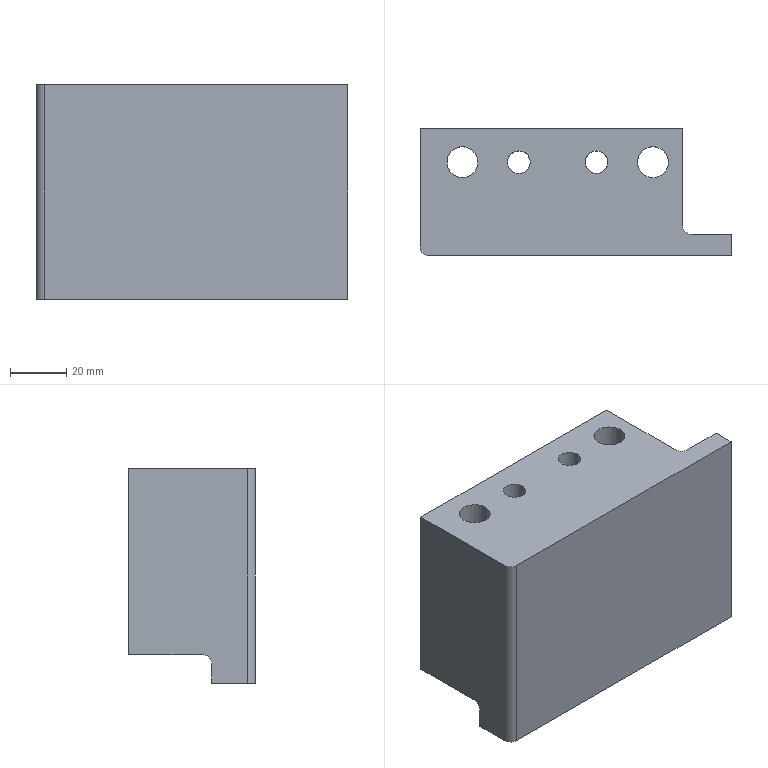Part | NX | features solid 2 | 1 solid | 25 faces | box 110.531 x 45 x 76 mm | volume 269432 mm3 | plane 14 | cylinder 11 | commonest cylinder face diameters 6 x3 8 x2 10.505 x2 11 x2 17 x2
STEP:
#1=CARTESIAN_POINT('',(682.498,166.969,32.999));
#2=VERTEX_POINT('',#1);
#3=CARTESIAN_POINT('',(682.498,201.487,32.999));
#4=VERTEX_POINT('',#3);
#5=CARTESIAN_POINT('',(682.498,196.487,32.999));
#6=DIRECTION('',(0.,-1.,-0.000000517));
#7=VECTOR('',#6,1000.);
#8=LINE('',#5,#7);
#9=EDGE_CURVE('',#2,#4,#8,.F.);
#10=ORIENTED_EDGE('',*,*,#9,.F.);
#11=CARTESIAN_POINT('',(682.498,166.969,-33.001));
#12=VERTEX_POINT('',#11);
#13=CARTESIAN_POINT('',(682.498,166.969,-43.001));
#14=DIRECTION('',(0.,0.000004945,-1.));
#15=VECTOR('',#14,1000.);
#16=LINE('',#13,#15);
#17=EDGE_CURVE('',#2,#12,#16,.T.);
#18=ORIENTED_EDGE('',*,*,#17,.T.);
#19=CARTESIAN_POINT('',(682.498,166.969,-43.001));
#20=VERTEX_POINT('',#19);
#21=CARTESIAN_POINT('',(682.498,166.969,-33.001));
#22=CARTESIAN_POINT('',(682.498,166.969,-36.334));
#23=CARTESIAN_POINT('',(682.498,166.969,-39.668));
#24=CARTESIAN_POINT('',(682.498,166.969,-43.001));
#25=B_SPLINE_CURVE_WITH_KNOTS('',3,(#21,#22,#23,#24),.UNSPECIFIED.,.F.,.F.,(4,4),(0.,1.),.UNSPECIFIED.);
#26=EDGE_CURVE('',#12,#20,#25,.T.);
#27=ORIENTED_EDGE('',*,*,#26,.T.);
#28=CARTESIAN_POINT('',(682.498,171.969,-43.001));
#29=VERTEX_POINT('',#28);
#30=CARTESIAN_POINT('',(682.498,166.969,-43.001));
#31=CARTESIAN_POINT('',(682.498,168.636,-43.001));
#32=CARTESIAN_POINT('',(682.498,170.302,-43.001));
#33=CARTESIAN_POINT('',(682.498,171.969,-43.001));
#34=B_SPLINE_CURVE_WITH_KNOTS('',3,(#30,#31,#32,#33),.UNSPECIFIED.,.F.,.F.,(4,4),(0.,1.),.UNSPECIFIED.);
#35=EDGE_CURVE('',#29,#20,#34,.F.);
#36=ORIENTED_EDGE('',*,*,#35,.F.);
#37=CARTESIAN_POINT('',(682.498,171.969,-36.001));
#38=VERTEX_POINT('',#37);
#39=CARTESIAN_POINT('',(682.498,171.969,-43.001));
#40=CARTESIAN_POINT('',(682.498,171.969,-40.668));
#41=CARTESIAN_POINT('',(682.498,171.969,-38.334));
#42=CARTESIAN_POINT('',(682.498,171.969,-36.001));
#43=B_SPLINE_CURVE_WITH_KNOTS('',3,(#39,#40,#41,#42),.UNSPECIFIED.,.F.,.F.,(4,4),(0.,0.7),.UNSPECIFIED.);
#44=EDGE_CURVE('',#38,#29,#43,.F.);
#45=ORIENTED_EDGE('',*,*,#44,.F.);
#46=CARTESIAN_POINT('',(682.498,174.969,-33.001));
#47=VERTEX_POINT('',#46);
#48=CARTESIAN_POINT('',(682.498,174.969,-36.001));
#49=DIRECTION('',(1.,0.,0.));
#50=DIRECTION('',(0.,1.,0.));
#51=AXIS2_PLACEMENT_3D('',#48,#49,#50);
#52=CIRCLE('',#51,3.);
#53=EDGE_CURVE('',#38,#47,#52,.F.);
#54=ORIENTED_EDGE('',*,*,#53,.T.);
#55=CARTESIAN_POINT('',(682.498,201.487,-33.001));
#56=VERTEX_POINT('',#55);
#57=CARTESIAN_POINT('',(682.498,119.199,-33.001));
#58=DIRECTION('',(0.,-1.,-0.000000517));
#59=VECTOR('',#58,1000.);
#60=LINE('',#57,#59);
#61=EDGE_CURVE('',#47,#56,#60,.F.);
#62=ORIENTED_EDGE('',*,*,#61,.T.);
#63=CARTESIAN_POINT('',(682.498,201.487,-43.001));
#64=DIRECTION('',(0.,-0.000000517,1.));
#65=VECTOR('',#64,1000.);
#66=LINE('',#63,#65);
#67=EDGE_CURVE('',#56,#4,#66,.T.);
#68=ORIENTED_EDGE('',*,*,#67,.T.);
#69=EDGE_LOOP('',(#10,#18,#27,#36,#45,#54,#62,#68));
#70=FACE_BOUND('',#69,.T.);
#71=CARTESIAN_POINT('',(682.498,185.969,49.2));
#72=DIRECTION('',(1.,0.,0.));
#73=DIRECTION('',(0.,-1.,-0.000004363));
#74=AXIS2_PLACEMENT_3D('',#71,#72,#73);
#75=PLANE('',#74);
#76=ADVANCED_FACE('',(#70),#75,.T.);
#77=CARTESIAN_POINT('',(671.977,197.987,-33.001));
#78=VERTEX_POINT('',#77);
#79=CARTESIAN_POINT('',(671.977,189.487,-33.001));
#80=DIRECTION('',(-0.000000053,0.000000517,-1.));
#81=DIRECTION('',(0.,1.,0.000000517));
#82=AXIS2_PLACEMENT_3D('',#79,#80,#81);
#83=CIRCLE('',#82,8.5);
#84=EDGE_CURVE('',#78,#78,#83,.F.);
#85=ORIENTED_EDGE('',*,*,#84,.T.);
#86=EDGE_LOOP('',(#85));
#87=FACE_BOUND('',#86,.T.);
#88=CARTESIAN_POINT('',(651.977,194.739,-33.001));
#89=VERTEX_POINT('',#88);
#90=CARTESIAN_POINT('',(651.977,189.487,-33.001));
#91=DIRECTION('',(-0.000000053,0.000000517,-1.));
#92=DIRECTION('',(0.,1.,0.000000517));
#93=AXIS2_PLACEMENT_3D('',#90,#91,#92);
#94=CIRCLE('',#93,5.253);
#95=EDGE_CURVE('',#89,#89,#94,.F.);
#96=ORIENTED_EDGE('',*,*,#95,.T.);
#97=EDGE_LOOP('',(#96));
#98=FACE_BOUND('',#97,.T.);
#99=CARTESIAN_POINT('',(624.446,194.739,-33.001));
#100=VERTEX_POINT('',#99);
#101=CARTESIAN_POINT('',(624.446,189.487,-33.001));
#102=DIRECTION('',(-0.000000053,0.000000517,-1.));
#103=DIRECTION('',(0.,1.,0.000000517));
#104=AXIS2_PLACEMENT_3D('',#101,#102,#103);
#105=CIRCLE('',#104,5.253);
#106=EDGE_CURVE('',#100,#100,#105,.F.);
#107=ORIENTED_EDGE('',*,*,#106,.T.);
#108=EDGE_LOOP('',(#107));
#109=FACE_BOUND('',#108,.T.);
#110=CARTESIAN_POINT('',(604.446,197.987,-33.001));
#111=VERTEX_POINT('',#110);
#112=CARTESIAN_POINT('',(604.446,189.487,-33.001));
#113=DIRECTION('',(-0.000000053,0.000000517,-1.));
#114=DIRECTION('',(0.,1.,0.000000517));
#115=AXIS2_PLACEMENT_3D('',#112,#113,#114);
#116=CIRCLE('',#115,8.5);
#117=EDGE_CURVE('',#111,#111,#116,.F.);
#118=ORIENTED_EDGE('',*,*,#117,.T.);
#119=EDGE_LOOP('',(#118));
#120=FACE_BOUND('',#119,.T.);
#121=ORIENTED_EDGE('',*,*,#61,.F.);
#122=CARTESIAN_POINT('',(589.446,174.969,-33.001));
#123=VERTEX_POINT('',#122);
#124=CARTESIAN_POINT('',(589.446,174.969,-33.001));
#125=DIRECTION('',(1.,0.,-0.000000053));
#126=VECTOR('',#125,1000.);
#127=LINE('',#124,#126);
#128=EDGE_CURVE('',#47,#123,#127,.F.);
#129=ORIENTED_EDGE('',*,*,#128,.T.);
#130=CARTESIAN_POINT('',(589.446,201.487,-33.001));
#131=VERTEX_POINT('',#130);
#132=CARTESIAN_POINT('',(589.446,119.199,-33.001));
#133=DIRECTION('',(0.,-1.,-0.000000517));
#134=VECTOR('',#133,1000.);
#135=LINE('',#132,#134);
#136=EDGE_CURVE('',#131,#123,#135,.T.);
#137=ORIENTED_EDGE('',*,*,#136,.F.);
#138=CARTESIAN_POINT('',(574.977,201.487,-33.001));
#139=DIRECTION('',(-1.,0.,0.000000053));
#140=VECTOR('',#139,1000.);
#141=LINE('',#138,#140);
#142=EDGE_CURVE('',#56,#131,#141,.T.);
#143=ORIENTED_EDGE('',*,*,#142,.F.);
#144=EDGE_LOOP('',(#121,#129,#137,#143));
#145=FACE_BOUND('',#144,.T.);
#146=CARTESIAN_POINT('',(574.977,119.199,-33.001));
#147=DIRECTION('',(-0.000000053,0.000000517,-1.));
#148=DIRECTION('',(1.,0.,-0.000000053));
#149=AXIS2_PLACEMENT_3D('',#146,#147,#148);
#150=PLANE('',#149);
#151=ADVANCED_FACE('',(#87,#98,#109,#120,#145),#150,.T.);
#152=CARTESIAN_POINT('',(699.977,163.969,32.999));
#153=VERTEX_POINT('',#152);
#154=CARTESIAN_POINT('',(685.498,163.969,32.999));
#155=VERTEX_POINT('',#154);
#156=CARTESIAN_POINT('',(704.737,163.969,32.999));
#157=DIRECTION('',(1.,0.,-0.000000053));
#158=VECTOR('',#157,1000.);
#159=LINE('',#156,#158);
#160=EDGE_CURVE('',#153,#155,#159,.F.);
#161=ORIENTED_EDGE('',*,*,#160,.T.);
#162=CARTESIAN_POINT('',(685.498,166.969,32.999));
#163=DIRECTION('',(0.000000053,-0.000000517,1.));
#164=DIRECTION('',(-0.01202,-0.9999,-0.000000516));
#165=AXIS2_PLACEMENT_3D('',#162,#163,#164);
#166=ELLIPSE('',#165,3.,3.);
#167=EDGE_CURVE('',#155,#2,#166,.F.);
#168=ORIENTED_EDGE('',*,*,#167,.T.);
#169=ORIENTED_EDGE('',*,*,#9,.T.);
#170=CARTESIAN_POINT('',(589.446,201.487,32.999));
#171=VERTEX_POINT('',#170);
#172=CARTESIAN_POINT('',(699.977,201.487,32.999));
#173=DIRECTION('',(-1.,0.,0.000000053));
#174=VECTOR('',#173,1000.);
#175=LINE('',#172,#174);
#176=EDGE_CURVE('',#171,#4,#175,.F.);
#177=ORIENTED_EDGE('',*,*,#176,.F.);
#178=CARTESIAN_POINT('',(589.446,159.487,32.999));
#179=VERTEX_POINT('',#178);
#180=CARTESIAN_POINT('',(589.446,186.487,32.999));
#181=DIRECTION('',(0.,-1.,-0.000000517));
#182=VECTOR('',#181,1000.);
#183=LINE('',#180,#182);
#184=EDGE_CURVE('',#179,#171,#183,.F.);
#185=ORIENTED_EDGE('',*,*,#184,.F.);
#186=CARTESIAN_POINT('',(592.446,156.487,32.999));
#187=VERTEX_POINT('',#186);
#188=CARTESIAN_POINT('',(592.446,159.487,32.999));
#189=DIRECTION('',(-0.000000053,0.000000517,-1.));
#190=DIRECTION('',(0.,-1.,-0.000000517));
#191=AXIS2_PLACEMENT_3D('',#188,#189,#190);
#192=CIRCLE('',#191,3.);
#193=EDGE_CURVE('',#179,#187,#192,.F.);
#194=ORIENTED_EDGE('',*,*,#193,.T.);
#195=CARTESIAN_POINT('',(699.977,156.487,32.999));
#196=VERTEX_POINT('',#195);
#197=CARTESIAN_POINT('',(699.977,156.487,32.999));
#198=DIRECTION('',(-1.,0.,0.000000053));
#199=VECTOR('',#198,1000.);
#200=LINE('',#197,#199);
#201=EDGE_CURVE('',#187,#196,#200,.F.);
#202=ORIENTED_EDGE('',*,*,#201,.T.);
#203=CARTESIAN_POINT('',(699.977,196.487,32.999));
#204=DIRECTION('',(0.,-1.,-0.000000517));
#205=VECTOR('',#204,1000.);
#206=LINE('',#203,#205);
#207=EDGE_CURVE('',#153,#196,#206,.T.);
#208=ORIENTED_EDGE('',*,*,#207,.F.);
#209=EDGE_LOOP('',(#161,#168,#169,#177,#185,#194,#202,#208));
#210=FACE_BOUND('',#209,.T.);
#211=CARTESIAN_POINT('',(671.977,183.987,32.999));
#212=VERTEX_POINT('',#211);
#213=CARTESIAN_POINT('',(671.977,189.487,32.999));
#214=DIRECTION('',(0.000000053,-0.000000517,1.));
#215=DIRECTION('',(0.,-1.,-0.000000517));
#216=AXIS2_PLACEMENT_3D('',#213,#214,#215);
#217=CIRCLE('',#216,5.5);
#218=EDGE_CURVE('',#212,#212,#217,.T.);
#219=ORIENTED_EDGE('',*,*,#218,.F.);
#220=EDGE_LOOP('',(#219));
#221=FACE_BOUND('',#220,.T.);
#222=CARTESIAN_POINT('',(651.977,193.487,32.999));
#223=VERTEX_POINT('',#222);
#224=CARTESIAN_POINT('',(651.977,189.487,32.999));
#225=DIRECTION('',(0.000000053,-0.000000517,1.));
#226=DIRECTION('',(0.,1.,0.000000517));
#227=AXIS2_PLACEMENT_3D('',#224,#225,#226);
#228=CIRCLE('',#227,4.);
#229=EDGE_CURVE('',#223,#223,#228,.T.);
#230=ORIENTED_EDGE('',*,*,#229,.F.);
#231=EDGE_LOOP('',(#230));
#232=FACE_BOUND('',#231,.T.);
#233=CARTESIAN_POINT('',(624.446,193.487,32.999));
#234=VERTEX_POINT('',#233);
#235=CARTESIAN_POINT('',(624.446,189.487,32.999));
#236=DIRECTION('',(0.000000053,-0.000000517,1.));
#237=DIRECTION('',(0.,1.,0.000000517));
#238=AXIS2_PLACEMENT_3D('',#235,#236,#237);
#239=CIRCLE('',#238,4.);
#240=EDGE_CURVE('',#234,#234,#239,.T.);
#241=ORIENTED_EDGE('',*,*,#240,.F.);
#242=EDGE_LOOP('',(#241));
#243=FACE_BOUND('',#242,.T.);
#244=CARTESIAN_POINT('',(604.446,183.987,32.999));
#245=VERTEX_POINT('',#244);
#246=CARTESIAN_POINT('',(604.446,189.487,32.999));
#247=DIRECTION('',(0.000000053,-0.000000517,1.));
#248=DIRECTION('',(0.,-1.,-0.000000517));
#249=AXIS2_PLACEMENT_3D('',#246,#247,#248);
#250=CIRCLE('',#249,5.5);
#251=EDGE_CURVE('',#245,#245,#250,.T.);
#252=ORIENTED_EDGE('',*,*,#251,.F.);
#253=EDGE_LOOP('',(#252));
#254=FACE_BOUND('',#253,.T.);
#255=CARTESIAN_POINT('',(699.977,196.487,32.999));
#256=DIRECTION('',(0.000000053,-0.000000517,1.));
#257=DIRECTION('',(1.,0.,-0.000000053));
#258=AXIS2_PLACEMENT_3D('',#255,#256,#257);
#259=PLANE('',#258);
#260=ADVANCED_FACE('',(#210,#221,#232,#243,#254),#259,.T.);
#261=CARTESIAN_POINT('',(589.446,171.969,-36.001));
#262=VERTEX_POINT('',#261);
#263=CARTESIAN_POINT('',(589.446,171.969,-43.001));
#264=VERTEX_POINT('',#263);
#265=CARTESIAN_POINT('',(589.446,171.969,-43.001));
#266=DIRECTION('',(-0.000000053,0.000001782,-1.));
#267=VECTOR('',#266,1000.);
#268=LINE('',#265,#267);
#269=EDGE_CURVE('',#262,#264,#268,.T.);
#270=ORIENTED_EDGE('',*,*,#269,.F.);
#271=CARTESIAN_POINT('',(682.498,171.969,-36.001));
#272=DIRECTION('',(1.,0.,-0.000000053));
#273=VECTOR('',#272,1000.);
#274=LINE('',#271,#273);
#275=EDGE_CURVE('',#262,#38,#274,.T.);
#276=ORIENTED_EDGE('',*,*,#275,.T.);
#277=ORIENTED_EDGE('',*,*,#44,.T.);
#278=CARTESIAN_POINT('',(704.737,171.969,-43.001));
#279=DIRECTION('',(-1.,0.,0.000000053));
#280=VECTOR('',#279,1000.);
#281=LINE('',#278,#280);
#282=EDGE_CURVE('',#29,#264,#281,.T.);
#283=ORIENTED_EDGE('',*,*,#282,.T.);
#284=EDGE_LOOP('',(#270,#276,#277,#283));
#285=FACE_BOUND('',#284,.T.);
#286=CARTESIAN_POINT('',(704.737,171.969,-5.001));
#287=DIRECTION('',(0.,1.,0.000001782));
#288=DIRECTION('',(0.,0.000001782,-1.));
#289=AXIS2_PLACEMENT_3D('',#286,#287,#288);
#290=PLANE('',#289);
#291=ADVANCED_FACE('',(#285),#290,.T.);
#292=CARTESIAN_POINT('',(592.446,156.487,-43.001));
#293=VERTEX_POINT('',#292);
#294=CARTESIAN_POINT('',(699.977,156.487,-43.001));
#295=VERTEX_POINT('',#294);
#296=CARTESIAN_POINT('',(574.977,156.487,-43.001));
#297=DIRECTION('',(1.,0.,-0.000000053));
#298=VECTOR('',#297,1000.);
#299=LINE('',#296,#298);
#300=EDGE_CURVE('',#293,#295,#299,.T.);
#301=ORIENTED_EDGE('',*,*,#300,.T.);
#302=CARTESIAN_POINT('',(699.977,156.487,56.368));
#303=DIRECTION('',(0.000000053,-0.000000517,1.));
#304=VECTOR('',#303,1000.);
#305=LINE('',#302,#304);
#306=EDGE_CURVE('',#295,#196,#305,.T.);
#307=ORIENTED_EDGE('',*,*,#306,.T.);
#308=ORIENTED_EDGE('',*,*,#201,.F.);
#309=CARTESIAN_POINT('',(592.446,156.487,56.368));
#310=DIRECTION('',(-0.000000053,0.000000517,-1.));
#311=VECTOR('',#310,1000.);
#312=LINE('',#309,#311);
#313=EDGE_CURVE('',#187,#293,#312,.T.);
#314=ORIENTED_EDGE('',*,*,#313,.T.);
#315=EDGE_LOOP('',(#301,#307,#308,#314));
#316=FACE_BOUND('',#315,.T.);
#317=CARTESIAN_POINT('',(583.446,156.487,56.368));
#318=DIRECTION('',(0.,1.,0.000000517));
#319=DIRECTION('',(-0.000000053,0.000000517,-1.));
#320=AXIS2_PLACEMENT_3D('',#317,#318,#319);
#321=PLANE('',#320);
#322=ADVANCED_FACE('',(#316),#321,.F.);
#323=ORIENTED_EDGE('',*,*,#282,.F.);
#324=ORIENTED_EDGE('',*,*,#35,.T.);
#325=CARTESIAN_POINT('',(685.498,163.969,-43.001));
#326=VERTEX_POINT('',#325);
#327=CARTESIAN_POINT('',(685.498,166.969,-43.001));
#328=DIRECTION('',(-0.000000053,0.000000517,-1.));
#329=DIRECTION('',(-0.01202,-0.9999,-0.000000516));
#330=AXIS2_PLACEMENT_3D('',#327,#328,#329);
#331=ELLIPSE('',#330,3.,3.);
#332=EDGE_CURVE('',#20,#326,#331,.F.);
#333=ORIENTED_EDGE('',*,*,#332,.T.);
#334=CARTESIAN_POINT('',(699.977,163.969,-43.001));
#335=VERTEX_POINT('',#334);
#336=CARTESIAN_POINT('',(704.737,163.969,-43.001));
#337=DIRECTION('',(-1.,0.,0.000000053));
#338=VECTOR('',#337,1000.);
#339=LINE('',#336,#338);
#340=EDGE_CURVE('',#335,#326,#339,.T.);
#341=ORIENTED_EDGE('',*,*,#340,.F.);
#342=CARTESIAN_POINT('',(699.977,119.199,-43.001));
#343=DIRECTION('',(0.,1.,0.000000517));
#344=VECTOR('',#343,1000.);
#345=LINE('',#342,#344);
#346=EDGE_CURVE('',#295,#335,#345,.T.);
#347=ORIENTED_EDGE('',*,*,#346,.F.);
#348=ORIENTED_EDGE('',*,*,#300,.F.);
#349=CARTESIAN_POINT('',(589.446,159.487,-43.001));
#350=VERTEX_POINT('',#349);
#351=CARTESIAN_POINT('',(592.446,159.487,-43.001));
#352=DIRECTION('',(0.000000053,-0.000000517,1.));
#353=DIRECTION('',(0.,1.,0.000000517));
#354=AXIS2_PLACEMENT_3D('',#351,#352,#353);
#355=CIRCLE('',#354,3.);
#356=EDGE_CURVE('',#293,#350,#355,.F.);
#357=ORIENTED_EDGE('',*,*,#356,.T.);
#358=CARTESIAN_POINT('',(589.446,119.199,-43.001));
#359=DIRECTION('',(0.,-1.,-0.000000517));
#360=VECTOR('',#359,1000.);
#361=LINE('',#358,#360);
#362=EDGE_CURVE('',#264,#350,#361,.T.);
#363=ORIENTED_EDGE('',*,*,#362,.F.);
#364=EDGE_LOOP('',(#323,#324,#333,#341,#347,#348,#357,#363));
#365=FACE_BOUND('',#364,.T.);
#366=CARTESIAN_POINT('',(574.977,119.199,-43.001));
#367=DIRECTION('',(-0.000000053,0.000000517,-1.));
#368=DIRECTION('',(1.,0.,-0.000000053));
#369=AXIS2_PLACEMENT_3D('',#366,#367,#368);
#370=PLANE('',#369);
#371=ADVANCED_FACE('',(#365),#370,.T.);
#372=ORIENTED_EDGE('',*,*,#142,.T.);
#373=CARTESIAN_POINT('',(589.446,201.487,-43.001));
#374=DIRECTION('',(0.000000053,-0.000000517,1.));
#375=VECTOR('',#374,1000.);
#376=LINE('',#373,#375);
#377=EDGE_CURVE('',#171,#131,#376,.F.);
#378=ORIENTED_EDGE('',*,*,#377,.F.);
#379=ORIENTED_EDGE('',*,*,#176,.T.);
#380=ORIENTED_EDGE('',*,*,#67,.F.);
#381=EDGE_LOOP('',(#372,#378,#379,#380));
#382=FACE_BOUND('',#381,.T.);
#383=CARTESIAN_POINT('',(699.977,201.487,-43.001));
#384=DIRECTION('',(0.,1.,0.000000517));
#385=DIRECTION('',(-0.000000053,0.000000517,-1.));
#386=AXIS2_PLACEMENT_3D('',#383,#384,#385);
#387=PLANE('',#386);
#388=ADVANCED_FACE('',(#382),#387,.T.);
#389=ORIENTED_EDGE('',*,*,#136,.T.);
#390=CARTESIAN_POINT('',(589.446,174.969,-36.001));
#391=DIRECTION('',(-1.,0.,0.000000053));
#392=DIRECTION('',(0.000000053,0.,1.));
#393=AXIS2_PLACEMENT_3D('',#390,#391,#392);
#394=CIRCLE('',#393,3.);
#395=EDGE_CURVE('',#123,#262,#394,.F.);
#396=ORIENTED_EDGE('',*,*,#395,.T.);
#397=ORIENTED_EDGE('',*,*,#269,.T.);
#398=ORIENTED_EDGE('',*,*,#362,.T.);
#399=CARTESIAN_POINT('',(589.446,159.487,-43.001));
#400=DIRECTION('',(-0.000000053,0.000000517,-1.));
#401=VECTOR('',#400,1000.);
#402=LINE('',#399,#401);
#403=EDGE_CURVE('',#350,#179,#402,.F.);
#404=ORIENTED_EDGE('',*,*,#403,.T.);
#405=ORIENTED_EDGE('',*,*,#184,.T.);
#406=ORIENTED_EDGE('',*,*,#377,.T.);
#407=EDGE_LOOP('',(#389,#396,#397,#398,#404,#405,#406));
#408=FACE_BOUND('',#407,.T.);
#409=CARTESIAN_POINT('',(589.446,186.487,-43.001));
#410=DIRECTION('',(-1.,0.,0.000000053));
#411=DIRECTION('',(-0.000000053,0.000000517,-1.));
#412=AXIS2_PLACEMENT_3D('',#409,#410,#411);
#413=PLANE('',#412);
#414=ADVANCED_FACE('',(#408),#413,.T.);
#415=CARTESIAN_POINT('',(671.977,194.987,7.999));
#416=VERTEX_POINT('',#415);
#417=CARTESIAN_POINT('',(671.977,189.487,7.999));
#418=DIRECTION('',(-0.000000053,0.000000517,-1.));
#419=DIRECTION('',(0.,1.,0.000000517));
#420=AXIS2_PLACEMENT_3D('',#417,#418,#419);
#421=CIRCLE('',#420,5.5);
#422=EDGE_CURVE('',#416,#416,#421,.F.);
#423=ORIENTED_EDGE('',*,*,#422,.F.);
#424=EDGE_LOOP('',(#423));
#425=FACE_BOUND('',#424,.T.);
#426=ORIENTED_EDGE('',*,*,#218,.T.);
#427=EDGE_LOOP('',(#426));
#428=FACE_BOUND('',#427,.T.);
#429=CARTESIAN_POINT('',(671.977,189.487,33.999));
#430=DIRECTION('',(-0.000000053,0.000000517,-1.));
#431=DIRECTION('',(0.,1.,0.000000517));
#432=AXIS2_PLACEMENT_3D('',#429,#430,#431);
#433=CYLINDRICAL_SURFACE('',#432,5.5);
#434=ADVANCED_FACE('',(#425,#428),#433,.F.);
#435=ORIENTED_EDGE('',*,*,#84,.F.);
#436=EDGE_LOOP('',(#435));
#437=FACE_BOUND('',#436,.T.);
#438=CARTESIAN_POINT('',(671.977,197.987,7.999));
#439=VERTEX_POINT('',#438);
#440=CARTESIAN_POINT('',(671.977,189.487,7.999));
#441=DIRECTION('',(-0.000000053,0.000000517,-1.));
#442=DIRECTION('',(0.,1.,0.000000517));
#443=AXIS2_PLACEMENT_3D('',#440,#441,#442);
#444=CIRCLE('',#443,8.5);
#445=EDGE_CURVE('',#439,#439,#444,.T.);
#446=ORIENTED_EDGE('',*,*,#445,.F.);
#447=EDGE_LOOP('',(#446));
#448=FACE_BOUND('',#447,.T.);
#449=CARTESIAN_POINT('',(671.977,189.487,7.999));
#450=DIRECTION('',(-0.000000053,0.000000517,-1.));
#451=DIRECTION('',(0.,1.,0.000000517));
#452=AXIS2_PLACEMENT_3D('',#449,#450,#451);
#453=CYLINDRICAL_SURFACE('',#452,8.5);
#454=ADVANCED_FACE('',(#437,#448),#453,.F.);
#455=ORIENTED_EDGE('',*,*,#422,.T.);
#456=EDGE_LOOP('',(#455));
#457=FACE_BOUND('',#456,.T.);
#458=ORIENTED_EDGE('',*,*,#445,.T.);
#459=EDGE_LOOP('',(#458));
#460=FACE_BOUND('',#459,.T.);
#461=CARTESIAN_POINT('',(671.977,189.487,7.999));
#462=DIRECTION('',(-0.000000053,0.000000517,-1.));
#463=DIRECTION('',(0.,1.,0.000000517));
#464=AXIS2_PLACEMENT_3D('',#461,#462,#463);
#465=PLANE('',#464);
#466=ADVANCED_FACE('',(#457,#460),#465,.T.);
#467=CARTESIAN_POINT('',(655.977,189.487,-13.001));
#468=VERTEX_POINT('',#467);
#469=CARTESIAN_POINT('',(651.977,189.487,-13.001));
#470=DIRECTION('',(0.000000981,-0.000000517,-1.));
#471=DIRECTION('',(1.,0.,0.000000981));
#472=AXIS2_PLACEMENT_3D('',#469,#470,#471);
#473=CIRCLE('',#472,4.);
#474=EDGE_CURVE('',#468,#468,#473,.F.);
#475=ORIENTED_EDGE('',*,*,#474,.F.);
#476=EDGE_LOOP('',(#475));
#477=FACE_BOUND('',#476,.T.);
#478=ORIENTED_EDGE('',*,*,#229,.T.);
#479=EDGE_LOOP('',(#478));
#480=FACE_BOUND('',#479,.T.);
#481=CARTESIAN_POINT('',(651.977,189.487,33.999));
#482=DIRECTION('',(0.000000981,-0.000000517,-1.));
#483=DIRECTION('',(0.,1.,-0.000000517));
#484=AXIS2_PLACEMENT_3D('',#481,#482,#483);
#485=CYLINDRICAL_SURFACE('',#484,4.);
#486=ADVANCED_FACE('',(#477,#480),#485,.F.);
#487=ORIENTED_EDGE('',*,*,#95,.F.);
#488=EDGE_LOOP('',(#487));
#489=FACE_BOUND('',#488,.T.);
#490=CARTESIAN_POINT('',(657.23,189.487,-13.001));
#491=VERTEX_POINT('',#490);
#492=CARTESIAN_POINT('',(651.977,189.487,-13.001));
#493=DIRECTION('',(0.000000981,-0.000000517,-1.));
#494=DIRECTION('',(1.,0.,0.000000981));
#495=AXIS2_PLACEMENT_3D('',#492,#493,#494);
#496=CIRCLE('',#495,5.253);
#497=EDGE_CURVE('',#491,#491,#496,.T.);
#498=ORIENTED_EDGE('',*,*,#497,.F.);
#499=EDGE_LOOP('',(#498));
#500=FACE_BOUND('',#499,.T.);
#501=CARTESIAN_POINT('',(651.977,189.487,-33.001));
#502=DIRECTION('',(0.000000981,-0.000000517,-1.));
#503=DIRECTION('',(0.,1.,-0.000000517));
#504=AXIS2_PLACEMENT_3D('',#501,#502,#503);
#505=CYLINDRICAL_SURFACE('',#504,5.253);
#506=ADVANCED_FACE('',(#489,#500),#505,.F.);
#507=ORIENTED_EDGE('',*,*,#474,.T.);
#508=EDGE_LOOP('',(#507));
#509=FACE_BOUND('',#508,.T.);
#510=ORIENTED_EDGE('',*,*,#497,.T.);
#511=EDGE_LOOP('',(#510));
#512=FACE_BOUND('',#511,.T.);
#513=CARTESIAN_POINT('',(651.977,189.487,-13.001));
#514=DIRECTION('',(0.000000981,-0.000000517,-1.));
#515=DIRECTION('',(0.,1.,-0.000000517));
#516=AXIS2_PLACEMENT_3D('',#513,#514,#515);
#517=PLANE('',#516);
#518=ADVANCED_FACE('',(#509,#512),#517,.T.);
#519=CARTESIAN_POINT('',(624.446,193.487,-13.001));
#520=VERTEX_POINT('',#519);
#521=CARTESIAN_POINT('',(624.446,189.487,-13.001));
#522=DIRECTION('',(-0.000000981,-0.000000517,-1.));
#523=DIRECTION('',(0.,1.,-0.000000517));
#524=AXIS2_PLACEMENT_3D('',#521,#522,#523);
#525=CIRCLE('',#524,4.);
#526=EDGE_CURVE('',#520,#520,#525,.T.);
#527=ORIENTED_EDGE('',*,*,#526,.T.);
#528=EDGE_LOOP('',(#527));
#529=FACE_BOUND('',#528,.T.);
#530=ORIENTED_EDGE('',*,*,#240,.T.);
#531=EDGE_LOOP('',(#530));
#532=FACE_BOUND('',#531,.T.);
#533=CARTESIAN_POINT('',(624.446,189.487,33.999));
#534=DIRECTION('',(-0.000000981,-0.000000517,-1.));
#535=DIRECTION('',(0.,1.,-0.000000517));
#536=AXIS2_PLACEMENT_3D('',#533,#534,#535);
#537=CYLINDRICAL_SURFACE('',#536,4.);
#538=ADVANCED_FACE('',(#529,#532),#537,.F.);
#539=ORIENTED_EDGE('',*,*,#106,.F.);
#540=EDGE_LOOP('',(#539));
#541=FACE_BOUND('',#540,.T.);
#542=CARTESIAN_POINT('',(619.194,189.487,-13.001));
#543=VERTEX_POINT('',#542);
#544=CARTESIAN_POINT('',(624.446,189.487,-13.001));
#545=DIRECTION('',(-0.000000981,-0.000000517,-1.));
#546=DIRECTION('',(-1.,0.,0.000000981));
#547=AXIS2_PLACEMENT_3D('',#544,#545,#546);
#548=CIRCLE('',#547,5.253);
#549=EDGE_CURVE('',#543,#543,#548,.F.);
#550=ORIENTED_EDGE('',*,*,#549,.T.);
#551=EDGE_LOOP('',(#550));
#552=FACE_BOUND('',#551,.T.);
#553=CARTESIAN_POINT('',(624.446,189.487,-33.001));
#554=DIRECTION('',(-0.000000981,-0.000000517,-1.));
#555=DIRECTION('',(0.,1.,-0.000000517));
#556=AXIS2_PLACEMENT_3D('',#553,#554,#555);
#557=CYLINDRICAL_SURFACE('',#556,5.253);
#558=ADVANCED_FACE('',(#541,#552),#557,.F.);
#559=ORIENTED_EDGE('',*,*,#526,.F.);
#560=EDGE_LOOP('',(#559));
#561=FACE_BOUND('',#560,.T.);
#562=ORIENTED_EDGE('',*,*,#549,.F.);
#563=EDGE_LOOP('',(#562));
#564=FACE_BOUND('',#563,.T.);
#565=CARTESIAN_POINT('',(624.446,189.487,-13.001));
#566=DIRECTION('',(-0.000000981,-0.000000517,-1.));
#567=DIRECTION('',(0.,1.,-0.000000517));
#568=AXIS2_PLACEMENT_3D('',#565,#566,#567);
#569=PLANE('',#568);
#570=ADVANCED_FACE('',(#561,#564),#569,.T.);
#571=CARTESIAN_POINT('',(604.446,194.987,7.999));
#572=VERTEX_POINT('',#571);
#573=CARTESIAN_POINT('',(604.446,189.487,7.999));
#574=DIRECTION('',(0.000000053,0.000000517,-1.));
#575=DIRECTION('',(0.,1.,0.000000517));
#576=AXIS2_PLACEMENT_3D('',#573,#574,#575);
#577=CIRCLE('',#576,5.5);
#578=EDGE_CURVE('',#572,#572,#577,.T.);
#579=ORIENTED_EDGE('',*,*,#578,.T.);
#580=EDGE_LOOP('',(#579));
#581=FACE_BOUND('',#580,.T.);
#582=ORIENTED_EDGE('',*,*,#251,.T.);
#583=EDGE_LOOP('',(#582));
#584=FACE_BOUND('',#583,.T.);
#585=CARTESIAN_POINT('',(604.446,189.487,33.999));
#586=DIRECTION('',(0.000000053,0.000000517,-1.));
#587=DIRECTION('',(0.,1.,0.000000517));
#588=AXIS2_PLACEMENT_3D('',#585,#586,#587);
#589=CYLINDRICAL_SURFACE('',#588,5.5);
#590=ADVANCED_FACE('',(#581,#584),#589,.F.);
#591=ORIENTED_EDGE('',*,*,#117,.F.);
#592=EDGE_LOOP('',(#591));
#593=FACE_BOUND('',#592,.T.);
#594=CARTESIAN_POINT('',(604.446,197.987,7.999));
#595=VERTEX_POINT('',#594);
#596=CARTESIAN_POINT('',(604.446,189.487,7.999));
#597=DIRECTION('',(0.000000053,0.000000517,-1.));
#598=DIRECTION('',(0.,1.,0.000000517));
#599=AXIS2_PLACEMENT_3D('',#596,#597,#598);
#600=CIRCLE('',#599,8.5);
#601=EDGE_CURVE('',#595,#595,#600,.F.);
#602=ORIENTED_EDGE('',*,*,#601,.T.);
#603=EDGE_LOOP('',(#602));
#604=FACE_BOUND('',#603,.T.);
#605=CARTESIAN_POINT('',(604.446,189.487,7.999));
#606=DIRECTION('',(0.000000053,0.000000517,-1.));
#607=DIRECTION('',(0.,1.,0.000000517));
#608=AXIS2_PLACEMENT_3D('',#605,#606,#607);
#609=CYLINDRICAL_SURFACE('',#608,8.5);
#610=ADVANCED_FACE('',(#593,#604),#609,.F.);
#611=ORIENTED_EDGE('',*,*,#578,.F.);
#612=EDGE_LOOP('',(#611));
#613=FACE_BOUND('',#612,.T.);
#614=ORIENTED_EDGE('',*,*,#601,.F.);
#615=EDGE_LOOP('',(#614));
#616=FACE_BOUND('',#615,.T.);
#617=CARTESIAN_POINT('',(604.446,189.487,7.999));
#618=DIRECTION('',(0.000000053,0.000000517,-1.));
#619=DIRECTION('',(0.,1.,0.000000517));
#620=AXIS2_PLACEMENT_3D('',#617,#618,#619);
#621=PLANE('',#620);
#622=ADVANCED_FACE('',(#613,#616),#621,.T.);
#623=ORIENTED_EDGE('',*,*,#193,.F.);
#624=ORIENTED_EDGE('',*,*,#403,.F.);
#625=ORIENTED_EDGE('',*,*,#356,.F.);
#626=ORIENTED_EDGE('',*,*,#313,.F.);
#627=EDGE_LOOP('',(#623,#624,#625,#626));
#628=FACE_BOUND('',#627,.T.);
#629=CARTESIAN_POINT('',(592.446,159.487,56.368));
#630=DIRECTION('',(-0.000000053,0.000000517,-1.));
#631=DIRECTION('',(0.,1.,0.000000517));
#632=AXIS2_PLACEMENT_3D('',#629,#630,#631);
#633=CYLINDRICAL_SURFACE('',#632,3.);
#634=ADVANCED_FACE('',(#628),#633,.T.);
#635=ORIENTED_EDGE('',*,*,#346,.T.);
#636=CARTESIAN_POINT('',(699.977,163.969,-43.001));
#637=DIRECTION('',(0.000000053,-0.000004945,1.));
#638=VECTOR('',#637,1000.);
#639=LINE('',#636,#638);
#640=EDGE_CURVE('',#335,#153,#639,.T.);
#641=ORIENTED_EDGE('',*,*,#640,.T.);
#642=ORIENTED_EDGE('',*,*,#207,.T.);
#643=ORIENTED_EDGE('',*,*,#306,.F.);
#644=EDGE_LOOP('',(#635,#641,#642,#643));
#645=FACE_BOUND('',#644,.T.);
#646=CARTESIAN_POINT('',(699.977,156.487,-43.001));
#647=DIRECTION('',(1.,0.,-0.000000053));
#648=DIRECTION('',(0.000000053,-0.000001034,1.));
#649=AXIS2_PLACEMENT_3D('',#646,#647,#648);
#650=PLANE('',#649);
#651=ADVANCED_FACE('',(#645),#650,.T.);
#652=ORIENTED_EDGE('',*,*,#340,.T.);
#653=CARTESIAN_POINT('',(685.498,163.969,32.999));
#654=DIRECTION('',(0.,0.000004945,-1.));
#655=VECTOR('',#654,1000.);
#656=LINE('',#653,#655);
#657=EDGE_CURVE('',#326,#155,#656,.F.);
#658=ORIENTED_EDGE('',*,*,#657,.T.);
#659=ORIENTED_EDGE('',*,*,#160,.F.);
#660=ORIENTED_EDGE('',*,*,#640,.F.);
#661=EDGE_LOOP('',(#652,#658,#659,#660));
#662=FACE_BOUND('',#661,.T.);
#663=CARTESIAN_POINT('',(704.737,163.969,-5.001));
#664=DIRECTION('',(0.,1.,0.000004945));
#665=DIRECTION('',(0.,0.000004945,-1.));
#666=AXIS2_PLACEMENT_3D('',#663,#664,#665);
#667=PLANE('',#666);
#668=ADVANCED_FACE('',(#662),#667,.T.);
#669=ORIENTED_EDGE('',*,*,#167,.F.);
#670=ORIENTED_EDGE('',*,*,#657,.F.);
#671=ORIENTED_EDGE('',*,*,#332,.F.);
#672=ORIENTED_EDGE('',*,*,#26,.F.);
#673=ORIENTED_EDGE('',*,*,#17,.F.);
#674=EDGE_LOOP('',(#669,#670,#671,#672,#673));
#675=FACE_BOUND('',#674,.T.);
#676=CARTESIAN_POINT('',(685.498,166.969,49.2));
#677=DIRECTION('',(0.,-0.000004945,1.));
#678=DIRECTION('',(0.,1.,0.000004945));
#679=AXIS2_PLACEMENT_3D('',#676,#677,#678);
#680=CYLINDRICAL_SURFACE('',#679,3.);
#681=ADVANCED_FACE('',(#675),#680,.F.);
#682=ORIENTED_EDGE('',*,*,#395,.F.);
#683=ORIENTED_EDGE('',*,*,#128,.F.);
#684=ORIENTED_EDGE('',*,*,#53,.F.);
#685=ORIENTED_EDGE('',*,*,#275,.F.);
#686=EDGE_LOOP('',(#682,#683,#684,#685));
#687=FACE_BOUND('',#686,.T.);
#688=CARTESIAN_POINT('',(704.737,174.969,-36.001));
#689=DIRECTION('',(-1.,0.,0.000000053));
#690=DIRECTION('',(0.000000053,0.,1.));
#691=AXIS2_PLACEMENT_3D('',#688,#689,#690);
#692=CYLINDRICAL_SURFACE('',#691,3.);
#693=ADVANCED_FACE('',(#687),#692,.F.);
#694=CLOSED_SHELL('',(#76,#151,#260,#291,#322,#371,#388,#414,#434,#454,#466,#486,#506,#518,#538,#558,#570,#590,#610,#622,#634,#651,#668,#681,#693));
#695=MANIFOLD_SOLID_BREP('',#694);
#696=(LENGTH_UNIT()NAMED_UNIT(*)SI_UNIT(.MILLI.,.METRE.));
#697=UNCERTAINTY_MEASURE_WITH_UNIT(LENGTH_MEASURE(0.0508),#696,'','');
#698=(NAMED_UNIT(*)PLANE_ANGLE_UNIT()SI_UNIT($,.RADIAN.));
#699=(NAMED_UNIT(*)SI_UNIT($,.STERADIAN.)SOLID_ANGLE_UNIT());
#700=(GEOMETRIC_REPRESENTATION_CONTEXT(3)GLOBAL_UNCERTAINTY_ASSIGNED_CONTEXT((#697))GLOBAL_UNIT_ASSIGNED_CONTEXT((#696,#698,#699))REPRESENTATION_CONTEXT('',''));
#701=ADVANCED_BREP_SHAPE_REPRESENTATION('',(#695),#700);